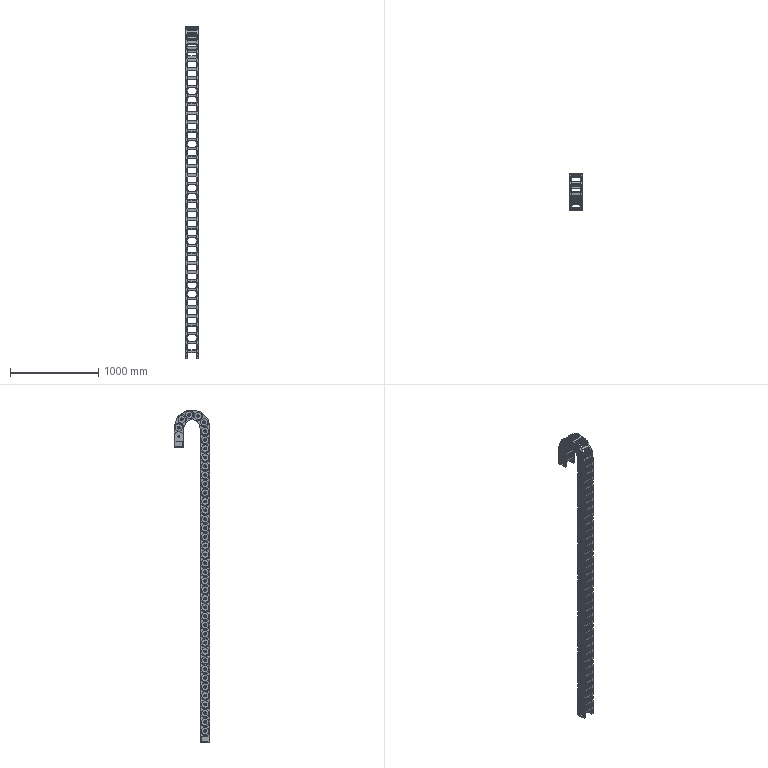Part | SolidWorks | 42 solids | 16536 faces | volume 15476828 mm3 | plane 8890 | cylinder 7646 | commonest cylinder face diameters 97 x1230 4 x492 47.5 x488 1 x480 81.7 x480 85.7 x480